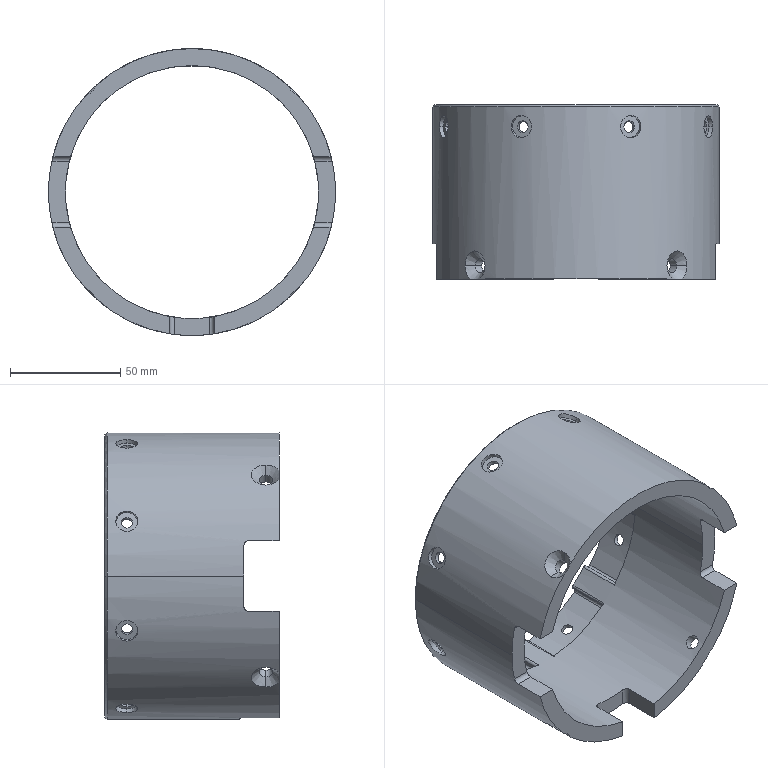Part | NX | features BREP 1 | 1 solid | 153 faces | box 130 x 79 x 130 mm | volume 198808 mm3 | cylinder 98 | plane 45 | cone 10 | commonest cylinder face diameters 2.2 x40 5.2 x16 10 x16 6.2 x8 122.2 x8 4 x6